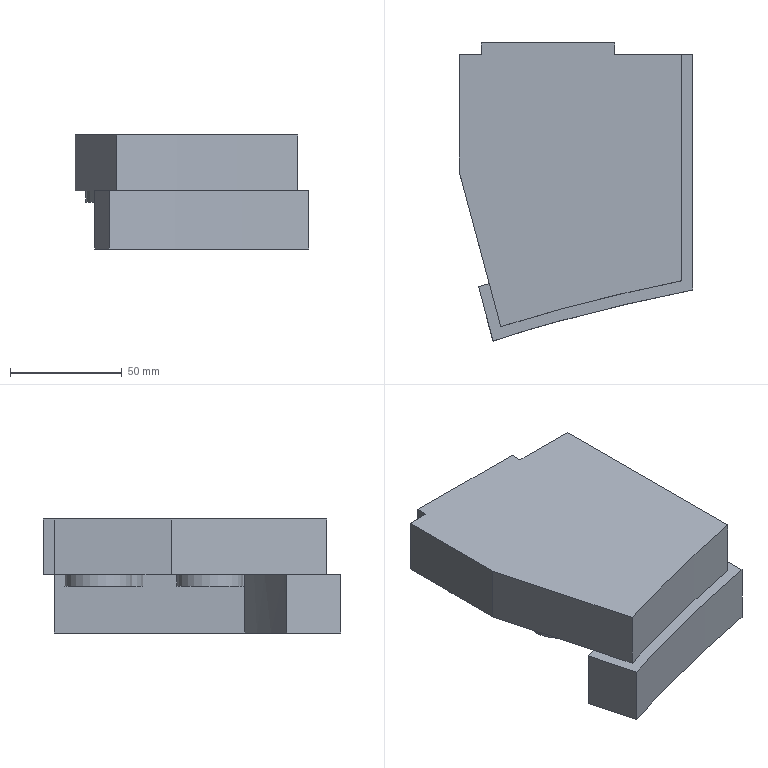Part | NX | features solid 2 | 1 solid | 26 faces | box 104.575 x 133.245 x 51 mm | volume 402266 mm3 | plane 19 | cylinder 4 | spline 3 | commonest cylinder face diameters 30 x4
STEP:
#1=CARTESIAN_POINT('',(-319.757,545.324,20.));
#2=VERTEX_POINT('',#1);
#3=CARTESIAN_POINT('',(-334.757,545.324,20.));
#4=DIRECTION('',(0.,0.,-1.));
#5=DIRECTION('',(1.,0.,0.));
#6=AXIS2_PLACEMENT_3D('',#3,#4,#5);
#7=CIRCLE('',#6,15.);
#8=EDGE_CURVE('',#2,#2,#7,.T.);
#9=ORIENTED_EDGE('',*,*,#8,.F.);
#10=EDGE_LOOP('',(#9));
#11=FACE_BOUND('',#10,.T.);
#12=CARTESIAN_POINT('',(-354.757,545.324,20.));
#13=VERTEX_POINT('',#12);
#14=CARTESIAN_POINT('',(-369.757,545.324,20.));
#15=DIRECTION('',(0.,0.,-1.));
#16=DIRECTION('',(1.,0.,0.));
#17=AXIS2_PLACEMENT_3D('',#14,#15,#16);
#18=CIRCLE('',#17,15.);
#19=EDGE_CURVE('',#13,#13,#18,.T.);
#20=ORIENTED_EDGE('',*,*,#19,.F.);
#21=EDGE_LOOP('',(#20));
#22=FACE_BOUND('',#21,.T.);
#23=CARTESIAN_POINT('',(-389.757,595.324,20.));
#24=VERTEX_POINT('',#23);
#25=CARTESIAN_POINT('',(-374.757,595.324,20.));
#26=DIRECTION('',(0.,0.,-1.));
#27=DIRECTION('',(-1.,0.,0.));
#28=AXIS2_PLACEMENT_3D('',#25,#26,#27);
#29=CIRCLE('',#28,15.);
#30=EDGE_CURVE('',#24,#24,#29,.F.);
#31=ORIENTED_EDGE('',*,*,#30,.T.);
#32=EDGE_LOOP('',(#31));
#33=FACE_BOUND('',#32,.T.);
#34=CARTESIAN_POINT('',(-354.757,590.324,20.));
#35=VERTEX_POINT('',#34);
#36=CARTESIAN_POINT('',(-339.757,590.324,20.));
#37=DIRECTION('',(0.,0.,-1.));
#38=DIRECTION('',(-1.,0.,0.));
#39=AXIS2_PLACEMENT_3D('',#36,#37,#38);
#40=CIRCLE('',#39,15.);
#41=EDGE_CURVE('',#35,#35,#40,.F.);
#42=ORIENTED_EDGE('',*,*,#41,.T.);
#43=EDGE_LOOP('',(#42));
#44=FACE_BOUND('',#43,.T.);
#45=CARTESIAN_POINT('',(-381.117,512.454,20.));
#46=VERTEX_POINT('',#45);
#47=CARTESIAN_POINT('',(-315.,529.858,20.));
#48=VERTEX_POINT('',#47);
#49=CARTESIAN_POINT('',(-385.887,510.936,20.));
#50=CARTESIAN_POINT('',(-384.617,511.345,20.));
#51=CARTESIAN_POINT('',(-364.232,517.853,20.));
#52=CARTESIAN_POINT('',(-332.141,526.365,20.));
#53=CARTESIAN_POINT('',(-301.295,532.824,20.));
#54=CARTESIAN_POINT('',(-290.,535.006,20.));
#55=B_SPLINE_CURVE_WITH_KNOTS('',3,(#49,#50,#51,#52,#53,#54),.UNSPECIFIED.,.F.,.F.,(4,1,1,4),(0.,0.04044,0.6485,1.),.UNSPECIFIED.);
#56=EDGE_CURVE('',#46,#48,#55,.T.);
#57=ORIENTED_EDGE('',*,*,#56,.F.);
#58=CARTESIAN_POINT('',(-394.575,562.679,20.));
#59=VERTEX_POINT('',#58);
#60=CARTESIAN_POINT('',(-371.65,477.121,20.));
#61=DIRECTION('',(0.2588,-0.9659,0.));
#62=VECTOR('',#61,1000.);
#63=LINE('',#60,#62);
#64=EDGE_CURVE('',#59,#46,#63,.T.);
#65=ORIENTED_EDGE('',*,*,#64,.F.);
#66=CARTESIAN_POINT('',(-394.575,615.,20.));
#67=VERTEX_POINT('',#66);
#68=CARTESIAN_POINT('',(-394.575,359.461,20.));
#69=DIRECTION('',(0.,1.,0.));
#70=VECTOR('',#69,1000.);
#71=LINE('',#68,#70);
#72=EDGE_CURVE('',#67,#59,#71,.F.);
#73=ORIENTED_EDGE('',*,*,#72,.F.);
#74=CARTESIAN_POINT('',(-384.575,615.,20.));
#75=VERTEX_POINT('',#74);
#76=CARTESIAN_POINT('',(-290.,615.,20.));
#77=DIRECTION('',(1.,0.,0.));
#78=VECTOR('',#77,1000.);
#79=LINE('',#76,#78);
#80=EDGE_CURVE('',#75,#67,#79,.F.);
#81=ORIENTED_EDGE('',*,*,#80,.F.);
#82=CARTESIAN_POINT('',(-384.575,620.,20.));
#83=VERTEX_POINT('',#82);
#84=CARTESIAN_POINT('',(-384.575,605.,20.));
#85=DIRECTION('',(0.,-1.,0.));
#86=VECTOR('',#85,1000.);
#87=LINE('',#84,#86);
#88=EDGE_CURVE('',#83,#75,#87,.T.);
#89=ORIENTED_EDGE('',*,*,#88,.F.);
#90=CARTESIAN_POINT('',(-325.,620.,20.));
#91=VERTEX_POINT('',#90);
#92=CARTESIAN_POINT('',(-290.,620.,20.));
#93=DIRECTION('',(1.,0.,0.));
#94=VECTOR('',#93,1000.);
#95=LINE('',#92,#94);
#96=EDGE_CURVE('',#91,#83,#95,.F.);
#97=ORIENTED_EDGE('',*,*,#96,.F.);
#98=CARTESIAN_POINT('',(-325.,615.,20.));
#99=VERTEX_POINT('',#98);
#100=CARTESIAN_POINT('',(-325.,605.,20.));
#101=DIRECTION('',(0.,-1.,0.));
#102=VECTOR('',#101,1000.);
#103=LINE('',#100,#102);
#104=EDGE_CURVE('',#91,#99,#103,.T.);
#105=ORIENTED_EDGE('',*,*,#104,.T.);
#106=CARTESIAN_POINT('',(-315.,615.,20.));
#107=VERTEX_POINT('',#106);
#108=CARTESIAN_POINT('',(-290.,615.,20.));
#109=DIRECTION('',(1.,0.,0.));
#110=VECTOR('',#109,1000.);
#111=LINE('',#108,#110);
#112=EDGE_CURVE('',#107,#99,#111,.F.);
#113=ORIENTED_EDGE('',*,*,#112,.F.);
#114=CARTESIAN_POINT('',(-315.,359.461,20.));
#115=DIRECTION('',(0.,1.,0.));
#116=VECTOR('',#115,1000.);
#117=LINE('',#114,#116);
#118=EDGE_CURVE('',#107,#48,#117,.F.);
#119=ORIENTED_EDGE('',*,*,#118,.T.);
#120=EDGE_LOOP('',(#57,#65,#73,#81,#89,#97,#105,#113,#119));
#121=FACE_BOUND('',#120,.T.);
#122=CARTESIAN_POINT('',(-561.977,359.461,20.));
#123=DIRECTION('',(0.,0.,-1.));
#124=DIRECTION('',(-1.,0.,0.));
#125=AXIS2_PLACEMENT_3D('',#122,#123,#124);
#126=PLANE('',#125);
#127=ADVANCED_FACE('',(#11,#22,#33,#44,#121),#126,.T.);
#128=CARTESIAN_POINT('',(-295.,513.633,20.));
#129=VERTEX_POINT('',#128);
#130=CARTESIAN_POINT('',(-375.936,493.117,20.));
#131=VERTEX_POINT('',#130);
#132=CARTESIAN_POINT('',(-295.,513.633,20.));
#133=CARTESIAN_POINT('',(-322.266,508.125,20.));
#134=CARTESIAN_POINT('',(-349.352,501.511,20.));
#135=CARTESIAN_POINT('',(-375.936,493.117,20.));
#136=B_SPLINE_CURVE_WITH_KNOTS('',3,(#132,#133,#134,#135),.UNSPECIFIED.,.F.,.F.,(4,4),(0.04428,0.9434),.UNSPECIFIED.);
#137=EDGE_CURVE('',#129,#131,#136,.T.);
#138=ORIENTED_EDGE('',*,*,#137,.T.);
#139=CARTESIAN_POINT('',(-371.65,477.121,20.));
#140=DIRECTION('',(0.2588,-0.9659,0.));
#141=VECTOR('',#140,1000.);
#142=LINE('',#139,#141);
#143=EDGE_CURVE('',#46,#131,#142,.T.);
#144=ORIENTED_EDGE('',*,*,#143,.F.);
#145=CARTESIAN_POINT('',(-385.887,510.936,20.));
#146=VERTEX_POINT('',#145);
#147=CARTESIAN_POINT('',(-385.887,510.936,20.));
#148=CARTESIAN_POINT('',(-384.617,511.345,20.));
#149=CARTESIAN_POINT('',(-364.232,517.853,20.));
#150=CARTESIAN_POINT('',(-332.141,526.365,20.));
#151=CARTESIAN_POINT('',(-301.295,532.824,20.));
#152=CARTESIAN_POINT('',(-290.,535.006,20.));
#153=B_SPLINE_CURVE_WITH_KNOTS('',3,(#147,#148,#149,#150,#151,#152),.UNSPECIFIED.,.F.,.F.,(4,1,1,4),(0.,0.04044,0.6485,1.),.UNSPECIFIED.);
#154=EDGE_CURVE('',#46,#146,#153,.F.);
#155=ORIENTED_EDGE('',*,*,#154,.T.);
#156=CARTESIAN_POINT('',(-379.408,486.755,20.));
#157=VERTEX_POINT('',#156);
#158=CARTESIAN_POINT('',(-359.814,413.63,20.));
#159=DIRECTION('',(0.2588,-0.9659,0.));
#160=VECTOR('',#159,1000.);
#161=LINE('',#158,#160);
#162=EDGE_CURVE('',#157,#146,#161,.F.);
#163=ORIENTED_EDGE('',*,*,#162,.F.);
#164=CARTESIAN_POINT('',(-290.,509.533,20.));
#165=VERTEX_POINT('',#164);
#166=CARTESIAN_POINT('',(-290.,509.533,20.));
#167=CARTESIAN_POINT('',(-299.448,507.664,20.));
#168=CARTESIAN_POINT('',(-327.896,501.626,20.));
#169=CARTESIAN_POINT('',(-357.656,493.733,20.));
#170=CARTESIAN_POINT('',(-377.786,487.282,20.));
#171=CARTESIAN_POINT('',(-379.408,486.755,20.));
#172=B_SPLINE_CURVE_WITH_KNOTS('',3,(#166,#167,#168,#169,#170,#171),.UNSPECIFIED.,.F.,.F.,(4,1,1,4),(0.,0.3128,0.9446,1.),.UNSPECIFIED.);
#173=EDGE_CURVE('',#157,#165,#172,.F.);
#174=ORIENTED_EDGE('',*,*,#173,.T.);
#175=CARTESIAN_POINT('',(-290.,615.,20.));
#176=VERTEX_POINT('',#175);
#177=CARTESIAN_POINT('',(-290.,359.461,20.));
#178=DIRECTION('',(0.,-1.,0.));
#179=VECTOR('',#178,1000.);
#180=LINE('',#177,#179);
#181=EDGE_CURVE('',#165,#176,#180,.F.);
#182=ORIENTED_EDGE('',*,*,#181,.T.);
#183=CARTESIAN_POINT('',(-295.,615.,20.));
#184=VERTEX_POINT('',#183);
#185=CARTESIAN_POINT('',(-561.977,615.,20.));
#186=DIRECTION('',(1.,0.,0.));
#187=VECTOR('',#186,1000.);
#188=LINE('',#185,#187);
#189=EDGE_CURVE('',#176,#184,#188,.F.);
#190=ORIENTED_EDGE('',*,*,#189,.T.);
#191=CARTESIAN_POINT('',(-295.,482.459,20.));
#192=DIRECTION('',(0.,1.,0.));
#193=VECTOR('',#192,1000.);
#194=LINE('',#191,#193);
#195=EDGE_CURVE('',#129,#184,#194,.T.);
#196=ORIENTED_EDGE('',*,*,#195,.F.);
#197=EDGE_LOOP('',(#138,#144,#155,#163,#174,#182,#190,#196));
#198=FACE_BOUND('',#197,.T.);
#199=CARTESIAN_POINT('',(-561.977,359.461,20.));
#200=DIRECTION('',(0.,0.,1.));
#201=DIRECTION('',(1.,0.,0.));
#202=AXIS2_PLACEMENT_3D('',#199,#200,#201);
#203=PLANE('',#202);
#204=ADVANCED_FACE('',(#198),#203,.T.);
#205=CARTESIAN_POINT('',(-394.575,615.,45.));
#206=VERTEX_POINT('',#205);
#207=CARTESIAN_POINT('',(-394.575,615.,50.));
#208=DIRECTION('',(0.,0.,-1.));
#209=VECTOR('',#208,1000.);
#210=LINE('',#207,#209);
#211=EDGE_CURVE('',#206,#67,#210,.T.);
#212=ORIENTED_EDGE('',*,*,#211,.F.);
#213=CARTESIAN_POINT('',(-384.575,615.,45.));
#214=VERTEX_POINT('',#213);
#215=CARTESIAN_POINT('',(-290.,615.,45.));
#216=DIRECTION('',(-1.,0.,0.));
#217=VECTOR('',#216,1000.);
#218=LINE('',#215,#217);
#219=EDGE_CURVE('',#214,#206,#218,.T.);
#220=ORIENTED_EDGE('',*,*,#219,.F.);
#221=CARTESIAN_POINT('',(-384.575,615.,50.));
#222=DIRECTION('',(0.,0.,-1.));
#223=VECTOR('',#222,1000.);
#224=LINE('',#221,#223);
#225=EDGE_CURVE('',#214,#75,#224,.T.);
#226=ORIENTED_EDGE('',*,*,#225,.T.);
#227=ORIENTED_EDGE('',*,*,#80,.T.);
#228=EDGE_LOOP('',(#212,#220,#226,#227));
#229=FACE_BOUND('',#228,.T.);
#230=CARTESIAN_POINT('',(-290.,615.,50.));
#231=DIRECTION('',(0.,-1.,0.));
#232=DIRECTION('',(0.,0.,-1.));
#233=AXIS2_PLACEMENT_3D('',#230,#231,#232);
#234=PLANE('',#233);
#235=ADVANCED_FACE('',(#229),#234,.F.);
#236=CARTESIAN_POINT('',(-394.575,562.679,45.));
#237=VERTEX_POINT('',#236);
#238=CARTESIAN_POINT('',(-375.936,493.117,45.));
#239=VERTEX_POINT('',#238);
#240=CARTESIAN_POINT('',(-371.65,477.121,45.));
#241=DIRECTION('',(-0.2588,0.9659,0.));
#242=VECTOR('',#241,1000.);
#243=LINE('',#240,#242);
#244=EDGE_CURVE('',#237,#239,#243,.F.);
#245=ORIENTED_EDGE('',*,*,#244,.T.);
#246=CARTESIAN_POINT('',(-295.,513.633,45.));
#247=VERTEX_POINT('',#246);
#248=CARTESIAN_POINT('',(-295.,513.633,45.));
#249=CARTESIAN_POINT('',(-322.266,508.125,45.));
#250=CARTESIAN_POINT('',(-349.352,501.511,45.));
#251=CARTESIAN_POINT('',(-375.936,493.117,45.));
#252=B_SPLINE_CURVE_WITH_KNOTS('',3,(#248,#249,#250,#251),.UNSPECIFIED.,.F.,.F.,(4,4),(0.04428,0.9434),.UNSPECIFIED.);
#253=EDGE_CURVE('',#247,#239,#252,.T.);
#254=ORIENTED_EDGE('',*,*,#253,.F.);
#255=CARTESIAN_POINT('',(-295.,615.,45.));
#256=VERTEX_POINT('',#255);
#257=CARTESIAN_POINT('',(-295.,-794.984,45.));
#258=DIRECTION('',(0.,1.,0.));
#259=VECTOR('',#258,1000.);
#260=LINE('',#257,#259);
#261=EDGE_CURVE('',#247,#256,#260,.T.);
#262=ORIENTED_EDGE('',*,*,#261,.T.);
#263=CARTESIAN_POINT('',(-325.,615.,45.));
#264=VERTEX_POINT('',#263);
#265=CARTESIAN_POINT('',(-290.,615.,45.));
#266=DIRECTION('',(-1.,0.,0.));
#267=VECTOR('',#266,1000.);
#268=LINE('',#265,#267);
#269=EDGE_CURVE('',#256,#264,#268,.T.);
#270=ORIENTED_EDGE('',*,*,#269,.T.);
#271=CARTESIAN_POINT('',(-325.,620.,45.));
#272=VERTEX_POINT('',#271);
#273=CARTESIAN_POINT('',(-325.,605.,45.));
#274=DIRECTION('',(0.,-1.,0.));
#275=VECTOR('',#274,1000.);
#276=LINE('',#273,#275);
#277=EDGE_CURVE('',#272,#264,#276,.T.);
#278=ORIENTED_EDGE('',*,*,#277,.F.);
#279=CARTESIAN_POINT('',(-384.575,620.,45.));
#280=VERTEX_POINT('',#279);
#281=CARTESIAN_POINT('',(-290.,620.,45.));
#282=DIRECTION('',(-1.,0.,0.));
#283=VECTOR('',#282,1000.);
#284=LINE('',#281,#283);
#285=EDGE_CURVE('',#272,#280,#284,.T.);
#286=ORIENTED_EDGE('',*,*,#285,.T.);
#287=CARTESIAN_POINT('',(-384.575,605.,45.));
#288=DIRECTION('',(0.,-1.,0.));
#289=VECTOR('',#288,1000.);
#290=LINE('',#287,#289);
#291=EDGE_CURVE('',#280,#214,#290,.T.);
#292=ORIENTED_EDGE('',*,*,#291,.T.);
#293=ORIENTED_EDGE('',*,*,#219,.T.);
#294=CARTESIAN_POINT('',(-394.575,-794.984,45.));
#295=DIRECTION('',(0.,-1.,0.));
#296=VECTOR('',#295,1000.);
#297=LINE('',#294,#296);
#298=EDGE_CURVE('',#206,#237,#297,.T.);
#299=ORIENTED_EDGE('',*,*,#298,.T.);
#300=EDGE_LOOP('',(#245,#254,#262,#270,#278,#286,#292,#293,#299));
#301=FACE_BOUND('',#300,.T.);
#302=CARTESIAN_POINT('',(-80.139,-794.984,45.));
#303=DIRECTION('',(0.,0.,1.));
#304=DIRECTION('',(1.,0.,0.));
#305=AXIS2_PLACEMENT_3D('',#302,#303,#304);
#306=PLANE('',#305);
#307=ADVANCED_FACE('',(#301),#306,.T.);
#308=ORIENTED_EDGE('',*,*,#64,.T.);
#309=ORIENTED_EDGE('',*,*,#143,.T.);
#310=CARTESIAN_POINT('',(-375.936,493.117,32.5));
#311=DIRECTION('',(0.,0.,1.));
#312=VECTOR('',#311,1000.);
#313=LINE('',#310,#312);
#314=EDGE_CURVE('',#131,#239,#313,.T.);
#315=ORIENTED_EDGE('',*,*,#314,.T.);
#316=ORIENTED_EDGE('',*,*,#244,.F.);
#317=CARTESIAN_POINT('',(-394.575,562.679,20.));
#318=DIRECTION('',(0.,0.,-1.));
#319=VECTOR('',#318,1000.);
#320=LINE('',#317,#319);
#321=EDGE_CURVE('',#237,#59,#320,.T.);
#322=ORIENTED_EDGE('',*,*,#321,.T.);
#323=EDGE_LOOP('',(#308,#309,#315,#316,#322));
#324=FACE_BOUND('',#323,.T.);
#325=CARTESIAN_POINT('',(-371.65,477.121,20.));
#326=DIRECTION('',(-0.9659,-0.2588,0.));
#327=DIRECTION('',(0.2588,-0.9659,0.));
#328=AXIS2_PLACEMENT_3D('',#325,#326,#327);
#329=PLANE('',#328);
#330=ADVANCED_FACE('',(#324),#329,.T.);
#331=ORIENTED_EDGE('',*,*,#112,.T.);
#332=CARTESIAN_POINT('',(-325.,615.,50.));
#333=DIRECTION('',(0.,0.,1.));
#334=VECTOR('',#333,1000.);
#335=LINE('',#332,#334);
#336=EDGE_CURVE('',#99,#264,#335,.T.);
#337=ORIENTED_EDGE('',*,*,#336,.T.);
#338=ORIENTED_EDGE('',*,*,#269,.F.);
#339=CARTESIAN_POINT('',(-295.,615.,50.));
#340=DIRECTION('',(0.,0.,1.));
#341=VECTOR('',#340,1000.);
#342=LINE('',#339,#341);
#343=EDGE_CURVE('',#184,#256,#342,.T.);
#344=ORIENTED_EDGE('',*,*,#343,.F.);
#345=ORIENTED_EDGE('',*,*,#189,.F.);
#346=CARTESIAN_POINT('',(-290.,615.,-6.));
#347=VERTEX_POINT('',#346);
#348=CARTESIAN_POINT('',(-290.,615.,50.));
#349=DIRECTION('',(0.,0.,-1.));
#350=VECTOR('',#349,1000.);
#351=LINE('',#348,#350);
#352=EDGE_CURVE('',#176,#347,#351,.T.);
#353=ORIENTED_EDGE('',*,*,#352,.T.);
#354=CARTESIAN_POINT('',(-315.,615.,-6.));
#355=VERTEX_POINT('',#354);
#356=CARTESIAN_POINT('',(-290.,615.,-6.));
#357=DIRECTION('',(-1.,0.,0.));
#358=VECTOR('',#357,1000.);
#359=LINE('',#356,#358);
#360=EDGE_CURVE('',#347,#355,#359,.T.);
#361=ORIENTED_EDGE('',*,*,#360,.T.);
#362=CARTESIAN_POINT('',(-315.,615.,50.));
#363=DIRECTION('',(0.,0.,-1.));
#364=VECTOR('',#363,1000.);
#365=LINE('',#362,#364);
#366=EDGE_CURVE('',#107,#355,#365,.T.);
#367=ORIENTED_EDGE('',*,*,#366,.F.);
#368=EDGE_LOOP('',(#331,#337,#338,#344,#345,#353,#361,#367));
#369=FACE_BOUND('',#368,.T.);
#370=CARTESIAN_POINT('',(-290.,615.,50.));
#371=DIRECTION('',(0.,-1.,0.));
#372=DIRECTION('',(0.,0.,-1.));
#373=AXIS2_PLACEMENT_3D('',#370,#371,#372);
#374=PLANE('',#373);
#375=ADVANCED_FACE('',(#369),#374,.F.);
#376=CARTESIAN_POINT('',(-315.,529.858,-6.));
#377=VERTEX_POINT('',#376);
#378=CARTESIAN_POINT('',(-315.,529.858,45.));
#379=DIRECTION('',(0.,0.,-1.));
#380=VECTOR('',#379,1000.);
#381=LINE('',#378,#380);
#382=EDGE_CURVE('',#48,#377,#381,.T.);
#383=ORIENTED_EDGE('',*,*,#382,.F.);
#384=ORIENTED_EDGE('',*,*,#118,.F.);
#385=ORIENTED_EDGE('',*,*,#366,.T.);
#386=CARTESIAN_POINT('',(-315.,467.794,-6.));
#387=DIRECTION('',(0.,1.,0.));
#388=VECTOR('',#387,1000.);
#389=LINE('',#386,#388);
#390=EDGE_CURVE('',#377,#355,#389,.T.);
#391=ORIENTED_EDGE('',*,*,#390,.F.);
#392=EDGE_LOOP('',(#383,#384,#385,#391));
#393=FACE_BOUND('',#392,.T.);
#394=CARTESIAN_POINT('',(-315.,467.794,50.));
#395=DIRECTION('',(-1.,0.,0.));
#396=DIRECTION('',(0.,0.,1.));
#397=AXIS2_PLACEMENT_3D('',#394,#395,#396);
#398=PLANE('',#397);
#399=ADVANCED_FACE('',(#393),#398,.T.);
#400=ORIENTED_EDGE('',*,*,#352,.F.);
#401=ORIENTED_EDGE('',*,*,#181,.F.);
#402=CARTESIAN_POINT('',(-290.,509.533,-6.));
#403=VERTEX_POINT('',#402);
#404=CARTESIAN_POINT('',(-290.,509.533,45.));
#405=DIRECTION('',(0.,0.,-1.));
#406=VECTOR('',#405,1000.);
#407=LINE('',#404,#406);
#408=EDGE_CURVE('',#165,#403,#407,.T.);
#409=ORIENTED_EDGE('',*,*,#408,.T.);
#410=CARTESIAN_POINT('',(-290.,-794.984,-6.));
#411=DIRECTION('',(0.,-1.,0.));
#412=VECTOR('',#411,1000.);
#413=LINE('',#410,#412);
#414=EDGE_CURVE('',#347,#403,#413,.T.);
#415=ORIENTED_EDGE('',*,*,#414,.F.);
#416=EDGE_LOOP('',(#400,#401,#409,#415));
#417=FACE_BOUND('',#416,.T.);
#418=CARTESIAN_POINT('',(-290.,600.,0.));
#419=DIRECTION('',(-1.,0.,0.));
#420=DIRECTION('',(0.,0.,1.));
#421=AXIS2_PLACEMENT_3D('',#418,#419,#420);
#422=PLANE('',#421);
#423=ADVANCED_FACE('',(#417),#422,.F.);
#424=ORIENTED_EDGE('',*,*,#162,.T.);
#425=CARTESIAN_POINT('',(-385.887,510.936,-6.));
#426=VERTEX_POINT('',#425);
#427=CARTESIAN_POINT('',(-385.887,510.936,45.));
#428=DIRECTION('',(0.,0.,-1.));
#429=VECTOR('',#428,1000.);
#430=LINE('',#427,#429);
#431=EDGE_CURVE('',#146,#426,#430,.T.);
#432=ORIENTED_EDGE('',*,*,#431,.T.);
#433=CARTESIAN_POINT('',(-379.408,486.755,-6.));
#434=VERTEX_POINT('',#433);
#435=CARTESIAN_POINT('',(-38.926,-783.941,-6.));
#436=DIRECTION('',(0.2588,-0.9659,0.));
#437=VECTOR('',#436,1000.);
#438=LINE('',#435,#437);
#439=EDGE_CURVE('',#426,#434,#438,.T.);
#440=ORIENTED_EDGE('',*,*,#439,.T.);
#441=CARTESIAN_POINT('',(-379.408,486.755,45.));
#442=DIRECTION('',(0.,0.,-1.));
#443=VECTOR('',#442,1000.);
#444=LINE('',#441,#443);
#445=EDGE_CURVE('',#157,#434,#444,.T.);
#446=ORIENTED_EDGE('',*,*,#445,.F.);
#447=EDGE_LOOP('',(#424,#432,#440,#446));
#448=FACE_BOUND('',#447,.T.);
#449=CARTESIAN_POINT('',(-409.752,600.,0.));
#450=DIRECTION('',(-0.9659,-0.2588,0.));
#451=DIRECTION('',(0.2588,-0.9659,0.));
#452=AXIS2_PLACEMENT_3D('',#449,#450,#451);
#453=PLANE('',#452);
#454=ADVANCED_FACE('',(#448),#453,.T.);
#455=CARTESIAN_POINT('',(-385.887,510.936,-6.));
#456=CARTESIAN_POINT('',(-384.617,511.345,-6.));
#457=CARTESIAN_POINT('',(-364.232,517.853,-6.));
#458=CARTESIAN_POINT('',(-332.141,526.365,-6.));
#459=CARTESIAN_POINT('',(-301.295,532.824,-6.));
#460=CARTESIAN_POINT('',(-290.,535.006,-6.));
#461=B_SPLINE_CURVE_WITH_KNOTS('',3,(#455,#456,#457,#458,#459,#460),.UNSPECIFIED.,.F.,.F.,(4,1,1,4),(0.,0.04044,0.6485,1.),.UNSPECIFIED.);
#462=EDGE_CURVE('',#426,#377,#461,.T.);
#463=ORIENTED_EDGE('',*,*,#462,.T.);
#464=ORIENTED_EDGE('',*,*,#390,.T.);
#465=ORIENTED_EDGE('',*,*,#360,.F.);
#466=ORIENTED_EDGE('',*,*,#414,.T.);
#467=CARTESIAN_POINT('',(-290.,509.533,-6.));
#468=CARTESIAN_POINT('',(-299.448,507.664,-6.));
#469=CARTESIAN_POINT('',(-327.896,501.626,-6.));
#470=CARTESIAN_POINT('',(-357.656,493.733,-6.));
#471=CARTESIAN_POINT('',(-377.786,487.282,-6.));
#472=CARTESIAN_POINT('',(-379.408,486.755,-6.));
#473=B_SPLINE_CURVE_WITH_KNOTS('',3,(#467,#468,#469,#470,#471,#472),.UNSPECIFIED.,.F.,.F.,(4,1,1,4),(0.,0.3128,0.9446,1.),.UNSPECIFIED.);
#474=EDGE_CURVE('',#403,#434,#473,.T.);
#475=ORIENTED_EDGE('',*,*,#474,.T.);
#476=ORIENTED_EDGE('',*,*,#439,.F.);
#477=EDGE_LOOP('',(#463,#464,#465,#466,#475,#476));
#478=FACE_BOUND('',#477,.T.);
#479=CARTESIAN_POINT('',(-80.139,-794.984,-6.));
#480=DIRECTION('',(0.,0.,1.));
#481=DIRECTION('',(1.,0.,0.));
#482=AXIS2_PLACEMENT_3D('',#479,#480,#481);
#483=PLANE('',#482);
#484=ADVANCED_FACE('',(#478),#483,.F.);
#485=ORIENTED_EDGE('',*,*,#343,.T.);
#486=ORIENTED_EDGE('',*,*,#261,.F.);
#487=CARTESIAN_POINT('',(-295.,513.633,32.5));
#488=DIRECTION('',(0.,0.,1.));
#489=VECTOR('',#488,1000.);
#490=LINE('',#487,#489);
#491=EDGE_CURVE('',#247,#129,#490,.F.);
#492=ORIENTED_EDGE('',*,*,#491,.T.);
#493=ORIENTED_EDGE('',*,*,#195,.T.);
#494=EDGE_LOOP('',(#485,#486,#492,#493));
#495=FACE_BOUND('',#494,.T.);
#496=CARTESIAN_POINT('',(-295.,482.459,20.));
#497=DIRECTION('',(1.,0.,0.));
#498=DIRECTION('',(0.,0.,-1.));
#499=AXIS2_PLACEMENT_3D('',#496,#497,#498);
#500=PLANE('',#499);
#501=ADVANCED_FACE('',(#495),#500,.T.);
#502=ORIENTED_EDGE('',*,*,#225,.F.);
#503=ORIENTED_EDGE('',*,*,#291,.F.);
#504=CARTESIAN_POINT('',(-384.575,620.,50.));
#505=DIRECTION('',(0.,0.,-1.));
#506=VECTOR('',#505,1000.);
#507=LINE('',#504,#506);
#508=EDGE_CURVE('',#280,#83,#507,.T.);
#509=ORIENTED_EDGE('',*,*,#508,.T.);
#510=ORIENTED_EDGE('',*,*,#88,.T.);
#511=EDGE_LOOP('',(#502,#503,#509,#510));
#512=FACE_BOUND('',#511,.T.);
#513=CARTESIAN_POINT('',(-384.575,605.,50.));
#514=DIRECTION('',(-1.,0.,0.));
#515=DIRECTION('',(0.,0.,1.));
#516=AXIS2_PLACEMENT_3D('',#513,#514,#515);
#517=PLANE('',#516);
#518=ADVANCED_FACE('',(#512),#517,.T.);
#519=ORIENTED_EDGE('',*,*,#336,.F.);
#520=ORIENTED_EDGE('',*,*,#104,.F.);
#521=CARTESIAN_POINT('',(-325.,620.,50.));
#522=DIRECTION('',(0.,0.,1.));
#523=VECTOR('',#522,1000.);
#524=LINE('',#521,#523);
#525=EDGE_CURVE('',#91,#272,#524,.T.);
#526=ORIENTED_EDGE('',*,*,#525,.T.);
#527=ORIENTED_EDGE('',*,*,#277,.T.);
#528=EDGE_LOOP('',(#519,#520,#526,#527));
#529=FACE_BOUND('',#528,.T.);
#530=CARTESIAN_POINT('',(-325.,605.,50.));
#531=DIRECTION('',(1.,0.,0.));
#532=DIRECTION('',(0.,0.,-1.));
#533=AXIS2_PLACEMENT_3D('',#530,#531,#532);
#534=PLANE('',#533);
#535=ADVANCED_FACE('',(#529),#534,.T.);
#536=ORIENTED_EDGE('',*,*,#508,.F.);
#537=ORIENTED_EDGE('',*,*,#285,.F.);
#538=ORIENTED_EDGE('',*,*,#525,.F.);
#539=ORIENTED_EDGE('',*,*,#96,.T.);
#540=EDGE_LOOP('',(#536,#537,#538,#539));
#541=FACE_BOUND('',#540,.T.);
#542=CARTESIAN_POINT('',(-290.,620.,50.));
#543=DIRECTION('',(0.,-1.,0.));
#544=DIRECTION('',(0.,0.,-1.));
#545=AXIS2_PLACEMENT_3D('',#542,#543,#544);
#546=PLANE('',#545);
#547=ADVANCED_FACE('',(#541),#546,.F.);
#548=CARTESIAN_POINT('',(-324.757,590.324,15.));
#549=VERTEX_POINT('',#548);
#550=CARTESIAN_POINT('',(-339.757,590.324,15.));
#551=DIRECTION('',(0.,0.,-1.));
#552=DIRECTION('',(1.,0.,0.));
#553=AXIS2_PLACEMENT_3D('',#550,#551,#552);
#554=CIRCLE('',#553,15.);
#555=EDGE_CURVE('',#549,#549,#554,.T.);
#556=ORIENTED_EDGE('',*,*,#555,.F.);
#557=EDGE_LOOP('',(#556));
#558=FACE_BOUND('',#557,.T.);
#559=ORIENTED_EDGE('',*,*,#41,.F.);
#560=EDGE_LOOP('',(#559));
#561=FACE_BOUND('',#560,.T.);
#562=CARTESIAN_POINT('',(-339.757,590.324,25.));
#563=DIRECTION('',(0.,0.,-1.));
#564=DIRECTION('',(-1.,0.,0.));
#565=AXIS2_PLACEMENT_3D('',#562,#563,#564);
#566=CYLINDRICAL_SURFACE('',#565,15.);
#567=ADVANCED_FACE('',(#558,#561),#566,.T.);
#568=ORIENTED_EDGE('',*,*,#555,.T.);
#569=EDGE_LOOP('',(#568));
#570=FACE_BOUND('',#569,.T.);
#571=CARTESIAN_POINT('',(-339.757,590.324,15.));
#572=DIRECTION('',(0.,0.,-1.));
#573=DIRECTION('',(-1.,0.,0.));
#574=AXIS2_PLACEMENT_3D('',#571,#572,#573);
#575=PLANE('',#574);
#576=ADVANCED_FACE('',(#570),#575,.T.);
#577=CARTESIAN_POINT('',(-359.757,595.324,15.));
#578=VERTEX_POINT('',#577);
#579=CARTESIAN_POINT('',(-374.757,595.324,15.));
#580=DIRECTION('',(0.,0.,-1.));
#581=DIRECTION('',(1.,0.,0.));
#582=AXIS2_PLACEMENT_3D('',#579,#580,#581);
#583=CIRCLE('',#582,15.);
#584=EDGE_CURVE('',#578,#578,#583,.T.);
#585=ORIENTED_EDGE('',*,*,#584,.F.);
#586=EDGE_LOOP('',(#585));
#587=FACE_BOUND('',#586,.T.);
#588=ORIENTED_EDGE('',*,*,#30,.F.);
#589=EDGE_LOOP('',(#588));
#590=FACE_BOUND('',#589,.T.);
#591=CARTESIAN_POINT('',(-374.757,595.324,25.));
#592=DIRECTION('',(0.,0.,-1.));
#593=DIRECTION('',(-1.,0.,0.));
#594=AXIS2_PLACEMENT_3D('',#591,#592,#593);
#595=CYLINDRICAL_SURFACE('',#594,15.);
#596=ADVANCED_FACE('',(#587,#590),#595,.T.);
#597=ORIENTED_EDGE('',*,*,#584,.T.);
#598=EDGE_LOOP('',(#597));
#599=FACE_BOUND('',#598,.T.);
#600=CARTESIAN_POINT('',(-374.757,595.324,15.));
#601=DIRECTION('',(0.,0.,-1.));
#602=DIRECTION('',(-1.,0.,0.));
#603=AXIS2_PLACEMENT_3D('',#600,#601,#602);
#604=PLANE('',#603);
#605=ADVANCED_FACE('',(#599),#604,.T.);
#606=ORIENTED_EDGE('',*,*,#298,.F.);
#607=ORIENTED_EDGE('',*,*,#211,.T.);
#608=ORIENTED_EDGE('',*,*,#72,.T.);
#609=ORIENTED_EDGE('',*,*,#321,.F.);
#610=EDGE_LOOP('',(#606,#607,#608,#609));
#611=FACE_BOUND('',#610,.T.);
#612=CARTESIAN_POINT('',(-394.575,645.,20.));
#613=DIRECTION('',(-1.,0.,0.));
#614=DIRECTION('',(0.,0.,1.));
#615=AXIS2_PLACEMENT_3D('',#612,#613,#614);
#616=PLANE('',#615);
#617=ADVANCED_FACE('',(#611),#616,.T.);
#618=ORIENTED_EDGE('',*,*,#154,.F.);
#619=ORIENTED_EDGE('',*,*,#56,.T.);
#620=ORIENTED_EDGE('',*,*,#382,.T.);
#621=ORIENTED_EDGE('',*,*,#462,.F.);
#622=ORIENTED_EDGE('',*,*,#431,.F.);
#623=EDGE_LOOP('',(#618,#619,#620,#621,#622));
#624=FACE_BOUND('',#623,.T.);
#625=CARTESIAN_POINT('',(-385.887,510.936,20.));
#626=CARTESIAN_POINT('',(-385.887,510.936,-6.));
#627=CARTESIAN_POINT('',(-362.635,518.434,20.));
#628=CARTESIAN_POINT('',(-362.635,518.434,-6.));
#629=CARTESIAN_POINT('',(-338.802,524.636,20.));
#630=CARTESIAN_POINT('',(-338.802,524.636,-6.));
#631=CARTESIAN_POINT('',(-315.,529.858,20.));
#632=CARTESIAN_POINT('',(-315.,529.858,-6.));
#633=B_SPLINE_SURFACE_WITH_KNOTS('',3,1,((#625,#626),(#627,#628),(#629,#630),(#631,#632)),.SURF_OF_LINEAR_EXTRUSION.,.F.,.F.,.F.,(4,4),(2,2),(0.,0.7407),(0.,1.),.PIECEWISE_BEZIER_KNOTS.);
#634=ADVANCED_FACE('',(#624),#633,.T.);
#635=ORIENTED_EDGE('',*,*,#173,.F.);
#636=ORIENTED_EDGE('',*,*,#445,.T.);
#637=ORIENTED_EDGE('',*,*,#474,.F.);
#638=ORIENTED_EDGE('',*,*,#408,.F.);
#639=EDGE_LOOP('',(#635,#636,#637,#638));
#640=FACE_BOUND('',#639,.T.);
#641=CARTESIAN_POINT('',(-290.,509.533,20.));
#642=CARTESIAN_POINT('',(-290.,509.533,-6.));
#643=CARTESIAN_POINT('',(-320.203,503.558,20.));
#644=CARTESIAN_POINT('',(-320.203,503.558,-6.));
#645=CARTESIAN_POINT('',(-350.15,496.254,20.));
#646=CARTESIAN_POINT('',(-350.15,496.254,-6.));
#647=CARTESIAN_POINT('',(-379.408,486.755,20.));
#648=CARTESIAN_POINT('',(-379.408,486.755,-6.));
#649=B_SPLINE_SURFACE_WITH_KNOTS('',3,1,((#641,#642),(#643,#644),(#645,#646),(#647,#648)),.SURF_OF_LINEAR_EXTRUSION.,.F.,.F.,.F.,(4,4),(2,2),(0.,1.),(0.,1.),.PIECEWISE_BEZIER_KNOTS.);
#650=ADVANCED_FACE('',(#640),#649,.T.);
#651=ORIENTED_EDGE('',*,*,#491,.F.);
#652=ORIENTED_EDGE('',*,*,#253,.T.);
#653=ORIENTED_EDGE('',*,*,#314,.F.);
#654=ORIENTED_EDGE('',*,*,#137,.F.);
#655=EDGE_LOOP('',(#651,#652,#653,#654));
#656=FACE_BOUND('',#655,.T.);
#657=CARTESIAN_POINT('',(-295.,513.633,20.));
#658=CARTESIAN_POINT('',(-295.,513.633,45.));
#659=CARTESIAN_POINT('',(-322.266,508.125,20.));
#660=CARTESIAN_POINT('',(-322.266,508.125,45.));
#661=CARTESIAN_POINT('',(-349.352,501.511,20.));
#662=CARTESIAN_POINT('',(-349.352,501.511,45.));
#663=CARTESIAN_POINT('',(-375.936,493.117,20.));
#664=CARTESIAN_POINT('',(-375.936,493.117,45.));
#665=B_SPLINE_SURFACE_WITH_KNOTS('',3,1,((#657,#658),(#659,#660),(#661,#662),(#663,#664)),.SURF_OF_LINEAR_EXTRUSION.,.F.,.F.,.F.,(4,4),(2,2),(0.04428,0.9434),(0.,1.),.PIECEWISE_BEZIER_KNOTS.);
#666=ADVANCED_FACE('',(#656),#665,.F.);
#667=ORIENTED_EDGE('',*,*,#19,.T.);
#668=EDGE_LOOP('',(#667));
#669=FACE_BOUND('',#668,.T.);
#670=CARTESIAN_POINT('',(-354.757,545.324,15.));
#671=VERTEX_POINT('',#670);
#672=CARTESIAN_POINT('',(-369.757,545.324,15.));
#673=DIRECTION('',(0.,0.,-1.));
#674=DIRECTION('',(1.,0.,0.));
#675=AXIS2_PLACEMENT_3D('',#672,#673,#674);
#676=CIRCLE('',#675,15.);
#677=EDGE_CURVE('',#671,#671,#676,.T.);
#678=ORIENTED_EDGE('',*,*,#677,.F.);
#679=EDGE_LOOP('',(#678));
#680=FACE_BOUND('',#679,.T.);
#681=CARTESIAN_POINT('',(-369.757,545.324,20.));
#682=DIRECTION('',(0.,0.,-1.));
#683=DIRECTION('',(-1.,0.,0.));
#684=AXIS2_PLACEMENT_3D('',#681,#682,#683);
#685=CYLINDRICAL_SURFACE('',#684,15.);
#686=ADVANCED_FACE('',(#669,#680),#685,.T.);
#687=ORIENTED_EDGE('',*,*,#677,.T.);
#688=EDGE_LOOP('',(#687));
#689=FACE_BOUND('',#688,.T.);
#690=CARTESIAN_POINT('',(-369.757,545.324,15.));
#691=DIRECTION('',(0.,0.,-1.));
#692=DIRECTION('',(-1.,0.,0.));
#693=AXIS2_PLACEMENT_3D('',#690,#691,#692);
#694=PLANE('',#693);
#695=ADVANCED_FACE('',(#689),#694,.T.);
#696=ORIENTED_EDGE('',*,*,#8,.T.);
#697=EDGE_LOOP('',(#696));
#698=FACE_BOUND('',#697,.T.);
#699=CARTESIAN_POINT('',(-319.757,545.324,15.));
#700=VERTEX_POINT('',#699);
#701=CARTESIAN_POINT('',(-334.757,545.324,15.));
#702=DIRECTION('',(0.,0.,-1.));
#703=DIRECTION('',(1.,0.,0.));
#704=AXIS2_PLACEMENT_3D('',#701,#702,#703);
#705=CIRCLE('',#704,15.);
#706=EDGE_CURVE('',#700,#700,#705,.T.);
#707=ORIENTED_EDGE('',*,*,#706,.F.);
#708=EDGE_LOOP('',(#707));
#709=FACE_BOUND('',#708,.T.);
#710=CARTESIAN_POINT('',(-334.757,545.324,20.));
#711=DIRECTION('',(0.,0.,-1.));
#712=DIRECTION('',(-1.,0.,0.));
#713=AXIS2_PLACEMENT_3D('',#710,#711,#712);
#714=CYLINDRICAL_SURFACE('',#713,15.);
#715=ADVANCED_FACE('',(#698,#709),#714,.T.);
#716=ORIENTED_EDGE('',*,*,#706,.T.);
#717=EDGE_LOOP('',(#716));
#718=FACE_BOUND('',#717,.T.);
#719=CARTESIAN_POINT('',(-334.757,545.324,15.));
#720=DIRECTION('',(0.,0.,-1.));
#721=DIRECTION('',(-1.,0.,0.));
#722=AXIS2_PLACEMENT_3D('',#719,#720,#721);
#723=PLANE('',#722);
#724=ADVANCED_FACE('',(#718),#723,.T.);
#725=CLOSED_SHELL('',(#127,#204,#235,#307,#330,#375,#399,#423,#454,#484,#501,#518,#535,#547,#567,#576,#596,#605,#617,#634,#650,#666,#686,#695,#715,#724));
#726=MANIFOLD_SOLID_BREP('',#725);
#727=(LENGTH_UNIT()NAMED_UNIT(*)SI_UNIT(.MILLI.,.METRE.));
#728=UNCERTAINTY_MEASURE_WITH_UNIT(LENGTH_MEASURE(0.0508),#727,'','');
#729=(NAMED_UNIT(*)PLANE_ANGLE_UNIT()SI_UNIT($,.RADIAN.));
#730=(NAMED_UNIT(*)SI_UNIT($,.STERADIAN.)SOLID_ANGLE_UNIT());
#731=(GEOMETRIC_REPRESENTATION_CONTEXT(3)GLOBAL_UNCERTAINTY_ASSIGNED_CONTEXT((#728))GLOBAL_UNIT_ASSIGNED_CONTEXT((#727,#729,#730))REPRESENTATION_CONTEXT('',''));
#732=ADVANCED_BREP_SHAPE_REPRESENTATION('',(#726),#731);